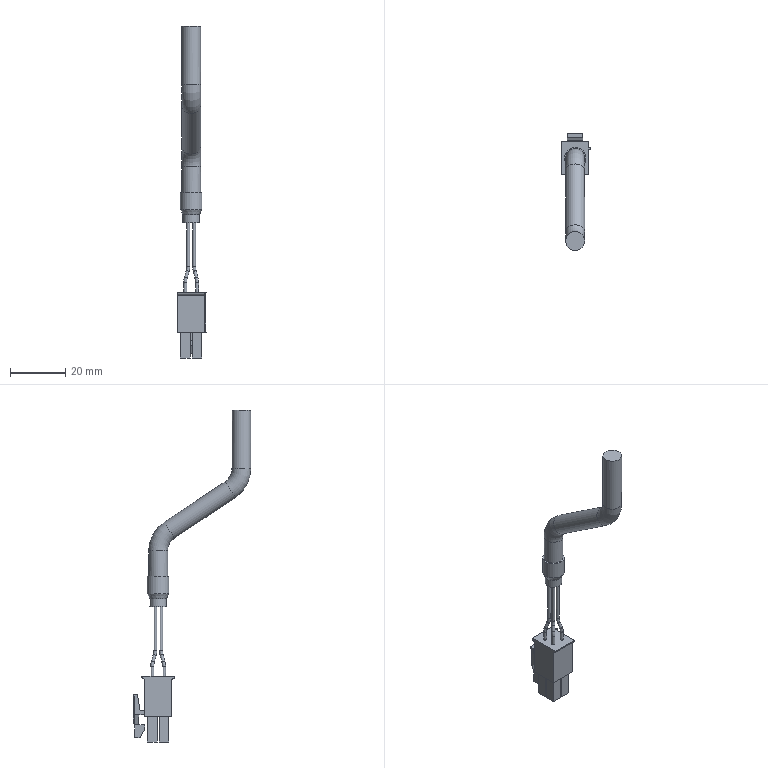Part | STEP file | 1 solid | 89 faces | box 10.4 x 42.4 x 119.7 mm | volume 5288 mm3 | plane 58 | cylinder 20 | torus 10 | cone 1 | commonest cylinder face diameters 1.1 x12 6.8 x3 1.6 x2 0.6 x1 6 x1 7.8 x1